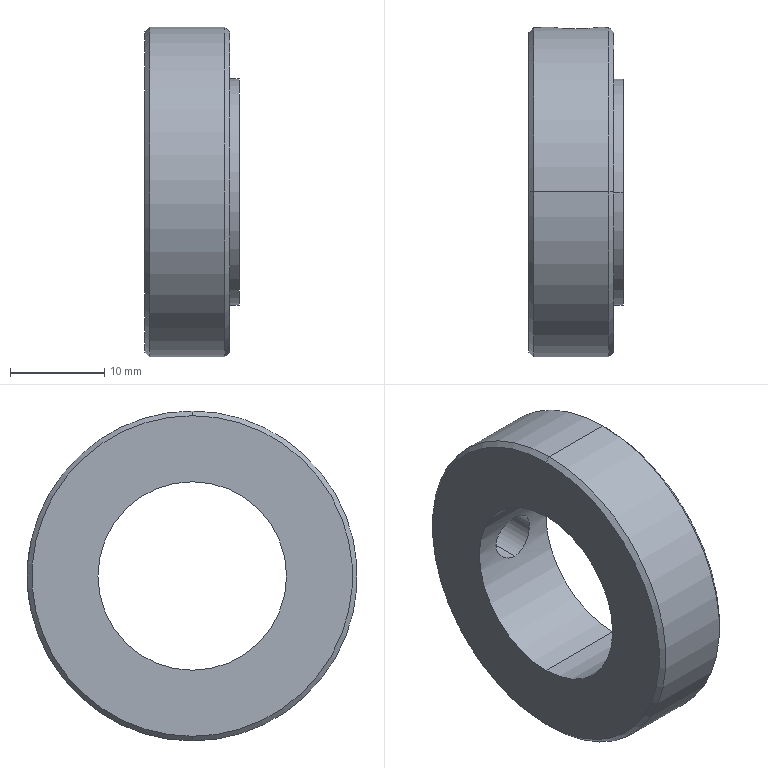Part | SolidWorks | features 3DProfileFeature 1, Chamfer 1, HoleWzd 1, Revolution 1 | 1 solid | 15 faces | box 10 x 35 x 35 mm | volume 5795 mm3 | cylinder 8 | cone 4 | plane 3 | commonest cylinder face diameters 5 x2 20 x2 24 x2 35 x2
STEP:
#1=CARTESIAN_POINT('',(9.,0.,-17.));
#2=VERTEX_POINT('',#1);
#3=CARTESIAN_POINT('',(9.,0.,17.));
#4=VERTEX_POINT('',#3);
#5=CARTESIAN_POINT('',(9.,0.,0.));
#6=DIRECTION('',(1.,0.,0.));
#7=DIRECTION('',(0.,0.,1.));
#8=AXIS2_PLACEMENT_3D('',#5,#6,#7);
#9=CIRCLE('',#8,17.);
#10=EDGE_CURVE('',#2,#4,#9,.T.);
#11=ORIENTED_EDGE('',*,*,#10,.F.);
#12=CARTESIAN_POINT('',(8.5,0.,-17.5));
#13=VERTEX_POINT('',#12);
#14=CARTESIAN_POINT('',(8.5,0.,-17.5));
#15=DIRECTION('',(-0.7071,0.,-0.7071));
#16=VECTOR('',#15,1000.);
#17=LINE('',#14,#16);
#18=EDGE_CURVE('',#2,#13,#17,.T.);
#19=ORIENTED_EDGE('',*,*,#18,.T.);
#20=CARTESIAN_POINT('',(8.5,0.,17.5));
#21=VERTEX_POINT('',#20);
#22=CARTESIAN_POINT('',(8.5,0.,0.));
#23=DIRECTION('',(-1.,0.,0.));
#24=DIRECTION('',(0.,0.,1.));
#25=AXIS2_PLACEMENT_3D('',#22,#23,#24);
#26=CIRCLE('',#25,17.5);
#27=EDGE_CURVE('',#21,#13,#26,.T.);
#28=ORIENTED_EDGE('',*,*,#27,.F.);
#29=CARTESIAN_POINT('',(8.5,0.,17.5));
#30=DIRECTION('',(-0.7071,0.,0.7071));
#31=VECTOR('',#30,1000.);
#32=LINE('',#29,#31);
#33=EDGE_CURVE('',#4,#21,#32,.T.);
#34=ORIENTED_EDGE('',*,*,#33,.F.);
#35=EDGE_LOOP('',(#11,#19,#28,#34));
#36=FACE_OUTER_BOUND('',#35,.T.);
#37=CARTESIAN_POINT('',(8.5,0.,0.));
#38=DIRECTION('',(-1.,0.,0.));
#39=DIRECTION('',(0.,0.,1.));
#40=AXIS2_PLACEMENT_3D('',#37,#38,#39);
#41=CONICAL_SURFACE('',#40,17.5,0.7854);
#42=ADVANCED_FACE('',(#36),#41,.T.);
#43=CARTESIAN_POINT('',(0.,0.,17.));
#44=VERTEX_POINT('',#43);
#45=CARTESIAN_POINT('',(0.,0.,-17.));
#46=VERTEX_POINT('',#45);
#47=CARTESIAN_POINT('',(0.,0.,0.));
#48=DIRECTION('',(-1.,0.,0.));
#49=DIRECTION('',(0.,0.,-1.));
#50=AXIS2_PLACEMENT_3D('',#47,#48,#49);
#51=CIRCLE('',#50,17.);
#52=EDGE_CURVE('',#44,#46,#51,.T.);
#53=ORIENTED_EDGE('',*,*,#52,.F.);
#54=CARTESIAN_POINT('',(0.5,0.,17.5));
#55=VERTEX_POINT('',#54);
#56=CARTESIAN_POINT('',(0.,0.,17.));
#57=DIRECTION('',(0.7071,0.,0.7071));
#58=VECTOR('',#57,1000.);
#59=LINE('',#56,#58);
#60=EDGE_CURVE('',#44,#55,#59,.T.);
#61=ORIENTED_EDGE('',*,*,#60,.T.);
#62=CARTESIAN_POINT('',(0.5,0.,-17.5));
#63=VERTEX_POINT('',#62);
#64=CARTESIAN_POINT('',(0.5,0.,0.));
#65=DIRECTION('',(1.,0.,0.));
#66=DIRECTION('',(0.,0.,-1.));
#67=AXIS2_PLACEMENT_3D('',#64,#65,#66);
#68=CIRCLE('',#67,17.5);
#69=EDGE_CURVE('',#63,#55,#68,.T.);
#70=ORIENTED_EDGE('',*,*,#69,.F.);
#71=CARTESIAN_POINT('',(0.,0.,-17.));
#72=DIRECTION('',(0.7071,0.,-0.7071));
#73=VECTOR('',#72,1000.);
#74=LINE('',#71,#73);
#75=EDGE_CURVE('',#46,#63,#74,.T.);
#76=ORIENTED_EDGE('',*,*,#75,.F.);
#77=EDGE_LOOP('',(#53,#61,#70,#76));
#78=FACE_OUTER_BOUND('',#77,.T.);
#79=CARTESIAN_POINT('',(0.,0.,0.));
#80=DIRECTION('',(1.,0.,0.));
#81=DIRECTION('',(0.,0.,-1.));
#82=AXIS2_PLACEMENT_3D('',#79,#80,#81);
#83=CONICAL_SURFACE('',#82,17.,0.7854);
#84=ADVANCED_FACE('',(#78),#83,.T.);
#85=CARTESIAN_POINT('',(5.,9.682,-2.5));
#86=VERTEX_POINT('',#85);
#87=CARTESIAN_POINT('',(5.,9.682,2.5));
#88=VERTEX_POINT('',#87);
#89=CARTESIAN_POINT('',(5.,9.682,-2.5));
#90=CARTESIAN_POINT('',(4.673,9.682,-2.5));
#91=CARTESIAN_POINT('',(4.343,9.7,-2.434));
#92=CARTESIAN_POINT('',(3.891,9.745,-2.247));
#93=CARTESIAN_POINT('',(3.745,9.763,-2.168));
#94=CARTESIAN_POINT('',(3.474,9.801,-1.987));
#95=CARTESIAN_POINT('',(3.348,9.822,-1.884));
#96=CARTESIAN_POINT('',(3.118,9.863,-1.653));
#97=CARTESIAN_POINT('',(3.013,9.884,-1.526));
#98=CARTESIAN_POINT('',(2.832,9.922,-1.255));
#99=CARTESIAN_POINT('',(2.755,9.939,-1.112));
#100=CARTESIAN_POINT('',(2.628,9.968,-0.808));
#101=CARTESIAN_POINT('',(2.581,9.98,-0.6507));
#102=CARTESIAN_POINT('',(2.517,9.996,-0.3307));
#103=CARTESIAN_POINT('',(2.5,10.,-0.1656));
#104=CARTESIAN_POINT('',(2.5,10.,0.1641));
#105=CARTESIAN_POINT('',(2.516,9.996,0.3268));
#106=CARTESIAN_POINT('',(2.58,9.98,0.6479));
#107=CARTESIAN_POINT('',(2.628,9.968,0.8075));
#108=CARTESIAN_POINT('',(2.754,9.939,1.109));
#109=CARTESIAN_POINT('',(2.83,9.922,1.253));
#110=CARTESIAN_POINT('',(3.012,9.884,1.525));
#111=CARTESIAN_POINT('',(3.117,9.863,1.652));
#112=CARTESIAN_POINT('',(3.346,9.822,1.882));
#113=CARTESIAN_POINT('',(3.473,9.801,1.986));
#114=CARTESIAN_POINT('',(3.745,9.763,2.168));
#115=CARTESIAN_POINT('',(3.888,9.745,2.245));
#116=CARTESIAN_POINT('',(4.189,9.715,2.371));
#117=CARTESIAN_POINT('',(4.349,9.703,2.419));
#118=CARTESIAN_POINT('',(4.671,9.687,2.484));
#119=CARTESIAN_POINT('',(4.834,9.682,2.5));
#120=CARTESIAN_POINT('',(5.,9.682,2.5));
#121=B_SPLINE_CURVE_WITH_KNOTS('',3,(#89,#90,#91,#92,#93,#94,#95,#96,#97,#98,#99,#100,#101,#102,#103,#104,#105,#106,#107,#108,#109,#110,#111,#112,#113,#114,#115,#116,#117,#118,#119,#120),.UNSPECIFIED.,.F.,.F.,(4,2,2,2,2,2,2,2,2,2,2,2,2,2,2,4),(0.007847,0.008828,0.009318,0.009809,0.0103,0.01079,0.01128,0.01177,0.01226,0.01275,0.01324,0.01373,0.01422,0.01471,0.0152,0.01569),.UNSPECIFIED.);
#122=EDGE_CURVE('',#86,#88,#121,.T.);
#123=ORIENTED_EDGE('',*,*,#122,.F.);
#124=CARTESIAN_POINT('',(5.,17.321,-2.5));
#125=VERTEX_POINT('',#124);
#126=CARTESIAN_POINT('',(5.,17.5,-2.5));
#127=DIRECTION('',(0.,1.,0.));
#128=VECTOR('',#127,1000.);
#129=LINE('',#126,#128);
#130=EDGE_CURVE('',#86,#125,#129,.T.);
#131=ORIENTED_EDGE('',*,*,#130,.T.);
#132=CARTESIAN_POINT('',(5.,17.321,2.5));
#133=VERTEX_POINT('',#132);
#134=CARTESIAN_POINT('',(5.,17.321,2.5));
#135=CARTESIAN_POINT('',(4.835,17.321,2.5));
#136=CARTESIAN_POINT('',(4.672,17.323,2.484));
#137=CARTESIAN_POINT('',(4.352,17.332,2.42));
#138=CARTESIAN_POINT('',(4.193,17.339,2.372));
#139=CARTESIAN_POINT('',(3.891,17.355,2.246));
#140=CARTESIAN_POINT('',(3.747,17.365,2.17));
#141=CARTESIAN_POINT('',(3.475,17.387,1.988));
#142=CARTESIAN_POINT('',(3.347,17.399,1.883));
#143=CARTESIAN_POINT('',(3.117,17.422,1.652));
#144=CARTESIAN_POINT('',(3.013,17.434,1.526));
#145=CARTESIAN_POINT('',(2.831,17.456,1.253));
#146=CARTESIAN_POINT('',(2.753,17.466,1.108));
#147=CARTESIAN_POINT('',(2.628,17.482,0.8072));
#148=CARTESIAN_POINT('',(2.58,17.489,0.6494));
#149=CARTESIAN_POINT('',(2.516,17.498,0.3266));
#150=CARTESIAN_POINT('',(2.5,17.5,0.1642));
#151=CARTESIAN_POINT('',(2.5,17.5,-0.1624));
#152=CARTESIAN_POINT('',(2.516,17.498,-0.3283));
#153=CARTESIAN_POINT('',(2.58,17.489,-0.6491));
#154=CARTESIAN_POINT('',(2.627,17.482,-0.805));
#155=CARTESIAN_POINT('',(2.753,17.466,-1.108));
#156=CARTESIAN_POINT('',(2.831,17.456,-1.254));
#157=CARTESIAN_POINT('',(3.012,17.434,-1.525));
#158=CARTESIAN_POINT('',(3.116,17.422,-1.651));
#159=CARTESIAN_POINT('',(3.349,17.399,-1.884));
#160=CARTESIAN_POINT('',(3.475,17.387,-1.987));
#161=CARTESIAN_POINT('',(3.745,17.365,-2.168));
#162=CARTESIAN_POINT('',(3.892,17.355,-2.247));
#163=CARTESIAN_POINT('',(4.194,17.339,-2.372));
#164=CARTESIAN_POINT('',(4.35,17.332,-2.42));
#165=CARTESIAN_POINT('',(4.671,17.323,-2.484));
#166=CARTESIAN_POINT('',(4.837,17.321,-2.5));
#167=CARTESIAN_POINT('',(5.,17.321,-2.5));
#168=B_SPLINE_CURVE_WITH_KNOTS('',3,(#134,#135,#136,#137,#138,#139,#140,#141,#142,#143,#144,#145,#146,#147,#148,#149,#150,#151,#152,#153,#154,#155,#156,#157,#158,#159,#160,#161,#162,#163,#164,#165,#166,#167),.UNSPECIFIED.,.F.,.F.,(4,2,2,2,2,2,2,2,2,2,2,2,2,2,2,2,4),(0.,0.0004891,0.0009783,0.001467,0.001957,0.002446,0.002935,0.003424,0.003913,0.004402,0.004891,0.00538,0.00587,0.006359,0.006848,0.007337,0.007826),.UNSPECIFIED.);
#169=EDGE_CURVE('',#133,#125,#168,.T.);
#170=ORIENTED_EDGE('',*,*,#169,.F.);
#171=CARTESIAN_POINT('',(5.,17.5,2.5));
#172=DIRECTION('',(0.,1.,0.));
#173=VECTOR('',#172,1000.);
#174=LINE('',#171,#173);
#175=EDGE_CURVE('',#88,#133,#174,.T.);
#176=ORIENTED_EDGE('',*,*,#175,.F.);
#177=EDGE_LOOP('',(#123,#131,#170,#176));
#178=FACE_OUTER_BOUND('',#177,.T.);
#179=CARTESIAN_POINT('',(5.,17.5,0.));
#180=DIRECTION('',(0.,1.,0.));
#181=DIRECTION('',(0.,0.,1.));
#182=AXIS2_PLACEMENT_3D('',#179,#180,#181);
#183=CYLINDRICAL_SURFACE('',#182,2.5);
#184=ADVANCED_FACE('',(#178),#183,.F.);
#185=CARTESIAN_POINT('',(10.,0.,-10.));
#186=VERTEX_POINT('',#185);
#187=CARTESIAN_POINT('',(10.,0.,10.));
#188=VERTEX_POINT('',#187);
#189=CARTESIAN_POINT('',(10.,0.,0.));
#190=DIRECTION('',(-1.,0.,0.));
#191=DIRECTION('',(0.,0.,1.));
#192=AXIS2_PLACEMENT_3D('',#189,#190,#191);
#193=CIRCLE('',#192,10.);
#194=EDGE_CURVE('',#186,#188,#193,.T.);
#195=ORIENTED_EDGE('',*,*,#194,.F.);
#196=CARTESIAN_POINT('',(0.,0.,-10.));
#197=VERTEX_POINT('',#196);
#198=CARTESIAN_POINT('',(0.,0.,-10.));
#199=DIRECTION('',(-1.,0.,0.));
#200=VECTOR('',#199,1000.);
#201=LINE('',#198,#200);
#202=EDGE_CURVE('',#186,#197,#201,.T.);
#203=ORIENTED_EDGE('',*,*,#202,.T.);
#204=CARTESIAN_POINT('',(0.,0.,10.));
#205=VERTEX_POINT('',#204);
#206=CARTESIAN_POINT('',(0.,0.,0.));
#207=DIRECTION('',(-1.,0.,0.));
#208=DIRECTION('',(0.,0.,1.));
#209=AXIS2_PLACEMENT_3D('',#206,#207,#208);
#210=CIRCLE('',#209,10.);
#211=EDGE_CURVE('',#197,#205,#210,.T.);
#212=ORIENTED_EDGE('',*,*,#211,.T.);
#213=CARTESIAN_POINT('',(0.,0.,10.));
#214=DIRECTION('',(-1.,0.,0.));
#215=VECTOR('',#214,1000.);
#216=LINE('',#213,#215);
#217=EDGE_CURVE('',#188,#205,#216,.T.);
#218=ORIENTED_EDGE('',*,*,#217,.F.);
#219=EDGE_LOOP('',(#195,#203,#212,#218));
#220=FACE_OUTER_BOUND('',#219,.T.);
#221=CARTESIAN_POINT('',(0.,0.,0.));
#222=DIRECTION('',(-1.,0.,0.));
#223=DIRECTION('',(0.,0.,1.));
#224=AXIS2_PLACEMENT_3D('',#221,#222,#223);
#225=CYLINDRICAL_SURFACE('',#224,10.);
#226=ADVANCED_FACE('',(#220),#225,.F.);
#227=CARTESIAN_POINT('',(10.,0.,12.));
#228=VERTEX_POINT('',#227);
#229=CARTESIAN_POINT('',(10.,0.,-12.));
#230=VERTEX_POINT('',#229);
#231=CARTESIAN_POINT('',(10.,0.,0.));
#232=DIRECTION('',(-1.,0.,0.));
#233=DIRECTION('',(0.,0.,1.));
#234=AXIS2_PLACEMENT_3D('',#231,#232,#233);
#235=CIRCLE('',#234,12.);
#236=EDGE_CURVE('',#228,#230,#235,.T.);
#237=ORIENTED_EDGE('',*,*,#236,.T.);
#238=CARTESIAN_POINT('',(9.,0.,-12.));
#239=VERTEX_POINT('',#238);
#240=CARTESIAN_POINT('',(0.,0.,-12.));
#241=DIRECTION('',(-1.,0.,0.));
#242=VECTOR('',#241,1000.);
#243=LINE('',#240,#242);
#244=EDGE_CURVE('',#230,#239,#243,.T.);
#245=ORIENTED_EDGE('',*,*,#244,.T.);
#246=CARTESIAN_POINT('',(9.,0.,12.));
#247=VERTEX_POINT('',#246);
#248=CARTESIAN_POINT('',(9.,0.,0.));
#249=DIRECTION('',(-1.,0.,0.));
#250=DIRECTION('',(0.,0.,1.));
#251=AXIS2_PLACEMENT_3D('',#248,#249,#250);
#252=CIRCLE('',#251,12.);
#253=EDGE_CURVE('',#247,#239,#252,.T.);
#254=ORIENTED_EDGE('',*,*,#253,.F.);
#255=CARTESIAN_POINT('',(0.,0.,12.));
#256=DIRECTION('',(-1.,0.,0.));
#257=VECTOR('',#256,1000.);
#258=LINE('',#255,#257);
#259=EDGE_CURVE('',#228,#247,#258,.T.);
#260=ORIENTED_EDGE('',*,*,#259,.F.);
#261=EDGE_LOOP('',(#237,#245,#254,#260));
#262=FACE_OUTER_BOUND('',#261,.T.);
#263=CARTESIAN_POINT('',(0.,0.,0.));
#264=DIRECTION('',(-1.,0.,0.));
#265=DIRECTION('',(0.,0.,1.));
#266=AXIS2_PLACEMENT_3D('',#263,#264,#265);
#267=CYLINDRICAL_SURFACE('',#266,12.);
#268=ADVANCED_FACE('',(#262),#267,.T.);
#269=ORIENTED_EDGE('',*,*,#169,.T.);
#270=CARTESIAN_POINT('',(5.,17.321,-2.5));
#271=CARTESIAN_POINT('',(5.163,17.321,-2.5));
#272=CARTESIAN_POINT('',(5.326,17.323,-2.484));
#273=CARTESIAN_POINT('',(5.649,17.332,-2.42));
#274=CARTESIAN_POINT('',(5.806,17.339,-2.372));
#275=CARTESIAN_POINT('',(6.107,17.355,-2.247));
#276=CARTESIAN_POINT('',(6.253,17.365,-2.17));
#277=CARTESIAN_POINT('',(6.526,17.387,-1.987));
#278=CARTESIAN_POINT('',(6.651,17.399,-1.884));
#279=CARTESIAN_POINT('',(6.882,17.422,-1.654));
#280=CARTESIAN_POINT('',(6.987,17.434,-1.525));
#281=CARTESIAN_POINT('',(7.169,17.456,-1.254));
#282=CARTESIAN_POINT('',(7.246,17.465,-1.111));
#283=CARTESIAN_POINT('',(7.371,17.482,-0.808));
#284=CARTESIAN_POINT('',(7.42,17.489,-0.6494));
#285=CARTESIAN_POINT('',(7.484,17.498,-0.3298));
#286=CARTESIAN_POINT('',(7.5,17.5,-0.1669));
#287=CARTESIAN_POINT('',(7.5,17.5,0.1636));
#288=CARTESIAN_POINT('',(7.484,17.498,0.3261));
#289=CARTESIAN_POINT('',(7.421,17.489,0.646));
#290=CARTESIAN_POINT('',(7.373,17.482,0.805));
#291=CARTESIAN_POINT('',(7.247,17.466,1.108));
#292=CARTESIAN_POINT('',(7.171,17.456,1.251));
#293=CARTESIAN_POINT('',(6.989,17.434,1.523));
#294=CARTESIAN_POINT('',(6.884,17.422,1.651));
#295=CARTESIAN_POINT('',(6.539,17.387,1.997));
#296=CARTESIAN_POINT('',(6.26,17.364,2.183));
#297=CARTESIAN_POINT('',(5.81,17.339,2.371));
#298=CARTESIAN_POINT('',(5.652,17.332,2.419));
#299=CARTESIAN_POINT('',(5.329,17.323,2.484));
#300=CARTESIAN_POINT('',(5.165,17.321,2.5));
#301=CARTESIAN_POINT('',(5.,17.321,2.5));
#302=B_SPLINE_CURVE_WITH_KNOTS('',3,(#270,#271,#272,#273,#274,#275,#276,#277,#278,#279,#280,#281,#282,#283,#284,#285,#286,#287,#288,#289,#290,#291,#292,#293,#294,#295,#296,#297,#298,#299,#300,#301),.UNSPECIFIED.,.F.,.F.,(4,2,2,2,2,2,2,2,2,2,2,2,2,2,2,4),(0.007826,0.008315,0.008804,0.009293,0.009782,0.01027,0.01076,0.01125,0.01174,0.01223,0.01272,0.01321,0.01369,0.01467,0.01516,0.01565),.UNSPECIFIED.);
#303=EDGE_CURVE('',#125,#133,#302,.T.);
#304=ORIENTED_EDGE('',*,*,#303,.T.);
#305=EDGE_LOOP('',(#269,#304));
#306=FACE_BOUND('',#305,.T.);
#307=ORIENTED_EDGE('',*,*,#27,.T.);
#308=CARTESIAN_POINT('',(0.,0.,-17.5));
#309=DIRECTION('',(-1.,0.,0.));
#310=VECTOR('',#309,1000.);
#311=LINE('',#308,#310);
#312=EDGE_CURVE('',#13,#63,#311,.T.);
#313=ORIENTED_EDGE('',*,*,#312,.T.);
#314=ORIENTED_EDGE('',*,*,#69,.T.);
#315=CARTESIAN_POINT('',(0.,0.,17.5));
#316=DIRECTION('',(-1.,0.,0.));
#317=VECTOR('',#316,1000.);
#318=LINE('',#315,#317);
#319=EDGE_CURVE('',#21,#55,#318,.T.);
#320=ORIENTED_EDGE('',*,*,#319,.F.);
#321=EDGE_LOOP('',(#307,#313,#314,#320));
#322=FACE_OUTER_BOUND('',#321,.T.);
#323=CARTESIAN_POINT('',(0.,0.,0.));
#324=DIRECTION('',(-1.,0.,0.));
#325=DIRECTION('',(0.,0.,1.));
#326=AXIS2_PLACEMENT_3D('',#323,#324,#325);
#327=CYLINDRICAL_SURFACE('',#326,17.5);
#328=ADVANCED_FACE('',(#306,#322),#327,.T.);
#329=CARTESIAN_POINT('',(0.,0.,0.));
#330=DIRECTION('',(-1.,0.,0.));
#331=DIRECTION('',(0.,0.,-1.));
#332=AXIS2_PLACEMENT_3D('',#329,#330,#331);
#333=CIRCLE('',#332,17.);
#334=EDGE_CURVE('',#46,#44,#333,.T.);
#335=ORIENTED_EDGE('',*,*,#334,.T.);
#336=ORIENTED_EDGE('',*,*,#52,.T.);
#337=EDGE_LOOP('',(#335,#336));
#338=FACE_OUTER_BOUND('',#337,.T.);
#339=CARTESIAN_POINT('',(0.,0.,0.));
#340=DIRECTION('',(-1.,0.,0.));
#341=DIRECTION('',(0.,0.,1.));
#342=AXIS2_PLACEMENT_3D('',#339,#340,#341);
#343=CIRCLE('',#342,10.);
#344=EDGE_CURVE('',#205,#197,#343,.T.);
#345=ORIENTED_EDGE('',*,*,#344,.F.);
#346=ORIENTED_EDGE('',*,*,#211,.F.);
#347=EDGE_LOOP('',(#345,#346));
#348=FACE_BOUND('',#347,.T.);
#349=CARTESIAN_POINT('',(0.,10.,0.));
#350=DIRECTION('',(1.,0.,0.));
#351=DIRECTION('',(0.,0.,-1.));
#352=AXIS2_PLACEMENT_3D('',#349,#350,#351);
#353=PLANE('',#352);
#354=ADVANCED_FACE('',(#338,#348),#353,.F.);
#355=ORIENTED_EDGE('',*,*,#312,.F.);
#356=CARTESIAN_POINT('',(8.5,0.,0.));
#357=DIRECTION('',(-1.,0.,0.));
#358=DIRECTION('',(0.,0.,1.));
#359=AXIS2_PLACEMENT_3D('',#356,#357,#358);
#360=CIRCLE('',#359,17.5);
#361=EDGE_CURVE('',#13,#21,#360,.T.);
#362=ORIENTED_EDGE('',*,*,#361,.T.);
#363=ORIENTED_EDGE('',*,*,#319,.T.);
#364=CARTESIAN_POINT('',(0.5,0.,0.));
#365=DIRECTION('',(1.,0.,0.));
#366=DIRECTION('',(0.,0.,-1.));
#367=AXIS2_PLACEMENT_3D('',#364,#365,#366);
#368=CIRCLE('',#367,17.5);
#369=EDGE_CURVE('',#55,#63,#368,.T.);
#370=ORIENTED_EDGE('',*,*,#369,.T.);
#371=EDGE_LOOP('',(#355,#362,#363,#370));
#372=FACE_OUTER_BOUND('',#371,.T.);
#373=CARTESIAN_POINT('',(0.,0.,0.));
#374=DIRECTION('',(-1.,0.,0.));
#375=DIRECTION('',(0.,0.,1.));
#376=AXIS2_PLACEMENT_3D('',#373,#374,#375);
#377=CYLINDRICAL_SURFACE('',#376,17.5);
#378=ADVANCED_FACE('',(#372),#377,.T.);
#379=CARTESIAN_POINT('',(9.,0.,0.));
#380=DIRECTION('',(1.,0.,0.));
#381=DIRECTION('',(0.,0.,1.));
#382=AXIS2_PLACEMENT_3D('',#379,#380,#381);
#383=CIRCLE('',#382,17.);
#384=EDGE_CURVE('',#4,#2,#383,.T.);
#385=ORIENTED_EDGE('',*,*,#384,.T.);
#386=ORIENTED_EDGE('',*,*,#10,.T.);
#387=EDGE_LOOP('',(#385,#386));
#388=FACE_OUTER_BOUND('',#387,.T.);
#389=ORIENTED_EDGE('',*,*,#253,.T.);
#390=CARTESIAN_POINT('',(9.,0.,0.));
#391=DIRECTION('',(-1.,0.,0.));
#392=DIRECTION('',(0.,0.,1.));
#393=AXIS2_PLACEMENT_3D('',#390,#391,#392);
#394=CIRCLE('',#393,12.);
#395=EDGE_CURVE('',#239,#247,#394,.T.);
#396=ORIENTED_EDGE('',*,*,#395,.T.);
#397=EDGE_LOOP('',(#389,#396));
#398=FACE_BOUND('',#397,.T.);
#399=CARTESIAN_POINT('',(9.,12.,0.));
#400=DIRECTION('',(-1.,0.,0.));
#401=DIRECTION('',(0.,0.,1.));
#402=AXIS2_PLACEMENT_3D('',#399,#400,#401);
#403=PLANE('',#402);
#404=ADVANCED_FACE('',(#388,#398),#403,.F.);
#405=ORIENTED_EDGE('',*,*,#244,.F.);
#406=CARTESIAN_POINT('',(10.,0.,0.));
#407=DIRECTION('',(-1.,0.,0.));
#408=DIRECTION('',(0.,0.,1.));
#409=AXIS2_PLACEMENT_3D('',#406,#407,#408);
#410=CIRCLE('',#409,12.);
#411=EDGE_CURVE('',#230,#228,#410,.T.);
#412=ORIENTED_EDGE('',*,*,#411,.T.);
#413=ORIENTED_EDGE('',*,*,#259,.T.);
#414=ORIENTED_EDGE('',*,*,#395,.F.);
#415=EDGE_LOOP('',(#405,#412,#413,#414));
#416=FACE_OUTER_BOUND('',#415,.T.);
#417=CARTESIAN_POINT('',(0.,0.,0.));
#418=DIRECTION('',(-1.,0.,0.));
#419=DIRECTION('',(0.,0.,1.));
#420=AXIS2_PLACEMENT_3D('',#417,#418,#419);
#421=CYLINDRICAL_SURFACE('',#420,12.);
#422=ADVANCED_FACE('',(#416),#421,.T.);
#423=ORIENTED_EDGE('',*,*,#236,.F.);
#424=ORIENTED_EDGE('',*,*,#411,.F.);
#425=EDGE_LOOP('',(#423,#424));
#426=FACE_OUTER_BOUND('',#425,.T.);
#427=CARTESIAN_POINT('',(10.,0.,0.));
#428=DIRECTION('',(-1.,0.,0.));
#429=DIRECTION('',(0.,0.,1.));
#430=AXIS2_PLACEMENT_3D('',#427,#428,#429);
#431=CIRCLE('',#430,10.);
#432=EDGE_CURVE('',#188,#186,#431,.T.);
#433=ORIENTED_EDGE('',*,*,#432,.T.);
#434=ORIENTED_EDGE('',*,*,#194,.T.);
#435=EDGE_LOOP('',(#433,#434));
#436=FACE_BOUND('',#435,.T.);
#437=CARTESIAN_POINT('',(10.,10.,0.));
#438=DIRECTION('',(-1.,0.,0.));
#439=DIRECTION('',(0.,0.,1.));
#440=AXIS2_PLACEMENT_3D('',#437,#438,#439);
#441=PLANE('',#440);
#442=ADVANCED_FACE('',(#426,#436),#441,.F.);
#443=ORIENTED_EDGE('',*,*,#202,.F.);
#444=ORIENTED_EDGE('',*,*,#432,.F.);
#445=ORIENTED_EDGE('',*,*,#217,.T.);
#446=ORIENTED_EDGE('',*,*,#344,.T.);
#447=EDGE_LOOP('',(#443,#444,#445,#446));
#448=FACE_OUTER_BOUND('',#447,.T.);
#449=CARTESIAN_POINT('',(5.,9.682,2.5));
#450=CARTESIAN_POINT('',(5.166,9.682,2.5));
#451=CARTESIAN_POINT('',(5.329,9.687,2.484));
#452=CARTESIAN_POINT('',(5.649,9.703,2.42));
#453=CARTESIAN_POINT('',(5.808,9.715,2.371));
#454=CARTESIAN_POINT('',(6.111,9.745,2.246));
#455=CARTESIAN_POINT('',(6.254,9.762,2.169));
#456=CARTESIAN_POINT('',(6.525,9.801,1.987));
#457=CARTESIAN_POINT('',(6.653,9.822,1.882));
#458=CARTESIAN_POINT('',(6.998,9.884,1.538));
#459=CARTESIAN_POINT('',(7.184,9.925,1.26));
#460=CARTESIAN_POINT('',(7.371,9.968,0.8089));
#461=CARTESIAN_POINT('',(7.419,9.98,0.6506));
#462=CARTESIAN_POINT('',(7.484,9.996,0.3275));
#463=CARTESIAN_POINT('',(7.5,10.,0.1648));
#464=CARTESIAN_POINT('',(7.5,10.,-0.1628));
#465=CARTESIAN_POINT('',(7.484,9.996,-0.3292));
#466=CARTESIAN_POINT('',(7.419,9.98,-0.6504));
#467=CARTESIAN_POINT('',(7.372,9.969,-0.8066));
#468=CARTESIAN_POINT('',(7.183,9.925,-1.262));
#469=CARTESIAN_POINT('',(6.999,9.884,-1.537));
#470=CARTESIAN_POINT('',(6.651,9.822,-1.884));
#471=CARTESIAN_POINT('',(6.526,9.801,-1.987));
#472=CARTESIAN_POINT('',(6.256,9.763,-2.168));
#473=CARTESIAN_POINT('',(6.109,9.745,-2.246));
#474=CARTESIAN_POINT('',(5.807,9.715,-2.372));
#475=CARTESIAN_POINT('',(5.652,9.703,-2.419));
#476=CARTESIAN_POINT('',(5.33,9.687,-2.484));
#477=CARTESIAN_POINT('',(5.164,9.682,-2.5));
#478=CARTESIAN_POINT('',(5.,9.682,-2.5));
#479=B_SPLINE_CURVE_WITH_KNOTS('',3,(#449,#450,#451,#452,#453,#454,#455,#456,#457,#458,#459,#460,#461,#462,#463,#464,#465,#466,#467,#468,#469,#470,#471,#472,#473,#474,#475,#476,#477,#478),.UNSPECIFIED.,.F.,.F.,(4,2,2,2,2,2,2,2,2,2,2,2,2,2,4),(0.,0.0004905,0.0009809,0.001471,0.001962,0.002943,0.003433,0.003924,0.004414,0.004905,0.005885,0.006376,0.006866,0.007357,0.007847),.UNSPECIFIED.);
#480=EDGE_CURVE('',#88,#86,#479,.T.);
#481=ORIENTED_EDGE('',*,*,#480,.T.);
#482=ORIENTED_EDGE('',*,*,#122,.T.);
#483=EDGE_LOOP('',(#481,#482));
#484=FACE_BOUND('',#483,.T.);
#485=CARTESIAN_POINT('',(0.,0.,0.));
#486=DIRECTION('',(-1.,0.,0.));
#487=DIRECTION('',(0.,0.,1.));
#488=AXIS2_PLACEMENT_3D('',#485,#486,#487);
#489=CYLINDRICAL_SURFACE('',#488,10.);
#490=ADVANCED_FACE('',(#448,#484),#489,.F.);
#491=ORIENTED_EDGE('',*,*,#130,.F.);
#492=ORIENTED_EDGE('',*,*,#480,.F.);
#493=ORIENTED_EDGE('',*,*,#175,.T.);
#494=ORIENTED_EDGE('',*,*,#303,.F.);
#495=EDGE_LOOP('',(#491,#492,#493,#494));
#496=FACE_OUTER_BOUND('',#495,.T.);
#497=CARTESIAN_POINT('',(5.,17.5,0.));
#498=DIRECTION('',(0.,1.,0.));
#499=DIRECTION('',(0.,0.,1.));
#500=AXIS2_PLACEMENT_3D('',#497,#498,#499);
#501=CYLINDRICAL_SURFACE('',#500,2.5);
#502=ADVANCED_FACE('',(#496),#501,.F.);
#503=ORIENTED_EDGE('',*,*,#60,.F.);
#504=ORIENTED_EDGE('',*,*,#334,.F.);
#505=ORIENTED_EDGE('',*,*,#75,.T.);
#506=ORIENTED_EDGE('',*,*,#369,.F.);
#507=EDGE_LOOP('',(#503,#504,#505,#506));
#508=FACE_OUTER_BOUND('',#507,.T.);
#509=CARTESIAN_POINT('',(0.,0.,0.));
#510=DIRECTION('',(1.,0.,0.));
#511=DIRECTION('',(0.,0.,-1.));
#512=AXIS2_PLACEMENT_3D('',#509,#510,#511);
#513=CONICAL_SURFACE('',#512,17.,0.7854);
#514=ADVANCED_FACE('',(#508),#513,.T.);
#515=ORIENTED_EDGE('',*,*,#18,.F.);
#516=ORIENTED_EDGE('',*,*,#384,.F.);
#517=ORIENTED_EDGE('',*,*,#33,.T.);
#518=ORIENTED_EDGE('',*,*,#361,.F.);
#519=EDGE_LOOP('',(#515,#516,#517,#518));
#520=FACE_OUTER_BOUND('',#519,.T.);
#521=CARTESIAN_POINT('',(8.5,0.,0.));
#522=DIRECTION('',(-1.,0.,0.));
#523=DIRECTION('',(0.,0.,1.));
#524=AXIS2_PLACEMENT_3D('',#521,#522,#523);
#525=CONICAL_SURFACE('',#524,17.5,0.7854);
#526=ADVANCED_FACE('',(#520),#525,.T.);
#527=CLOSED_SHELL('',(#42,#84,#184,#226,#268,#328,#354,#378,#404,#422,#442,#490,#502,#514,#526));
#528=MANIFOLD_SOLID_BREP('',#527);
#529=CARTESIAN_POINT('',(0.,0.,0.));
#530=DIRECTION('',(0.,0.,1.));
#531=DIRECTION('',(1.,0.,0.));
#532=AXIS2_PLACEMENT_3D('',#529,#530,#531);
#533=(LENGTH_UNIT()NAMED_UNIT(*)SI_UNIT(.MILLI.,.METRE.));
#534=UNCERTAINTY_MEASURE_WITH_UNIT(LENGTH_MEASURE(0.00001),#533,'','');
#535=(NAMED_UNIT(*)PLANE_ANGLE_UNIT()SI_UNIT($,.RADIAN.));
#536=(NAMED_UNIT(*)SI_UNIT($,.STERADIAN.)SOLID_ANGLE_UNIT());
#537=(GEOMETRIC_REPRESENTATION_CONTEXT(3)GLOBAL_UNCERTAINTY_ASSIGNED_CONTEXT((#534))GLOBAL_UNIT_ASSIGNED_CONTEXT((#533,#535,#536))REPRESENTATION_CONTEXT('',''));
#538=ADVANCED_BREP_SHAPE_REPRESENTATION('',(#528,#532),#537);